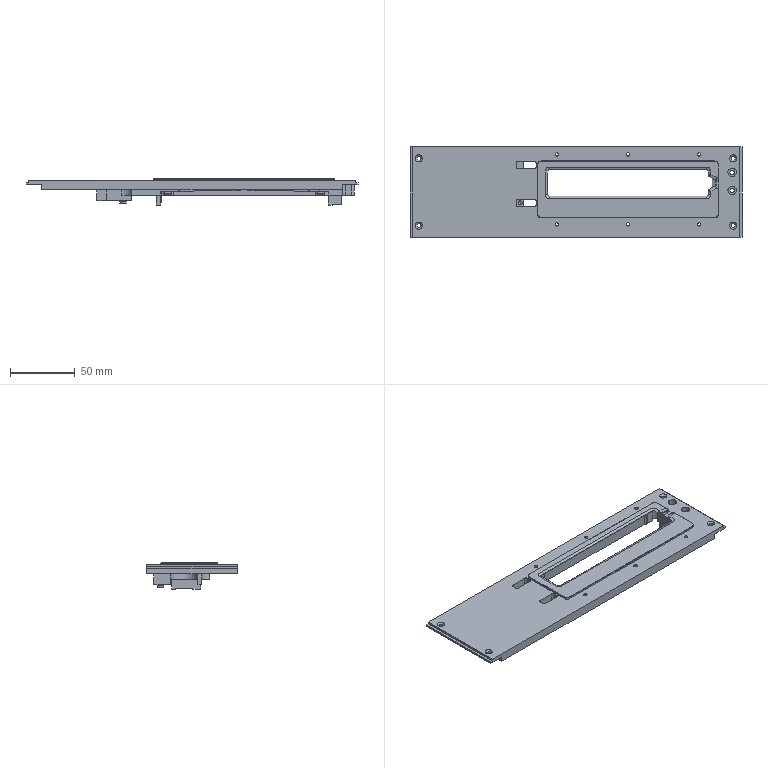NC program | NX | posted with a generic post | part box 256.6 x 70.3 x 20.422 mm
Lines 8840 to 9778 of 15201:
(HOLE_MILLING , TOOL : D3)
N17630 T03 M6
N17632 G54
N17634 G17 G0 G90 X120.7 Y15.17 S9500 M3
N17636 G43 Z30. H3
N17638 Z-0.9
N17640 G94 G3 X121.575 Y14.295 R0.875 F1250.
N17642 X122.45 Y15.17 R0.875
N17644 X122.45 Y15.17 Z-1.15 I-1.75 J0.
N17646 X122.45 Y15.17 Z-1.4 I-1.75 J0.
N17648 X122.45 Y15.17 Z-1.65 I-1.75 J0.
N17650 X122.45 Y15.17 Z-1.9 I-1.75 J0.
N17652 X122.45 Y15.17 Z-2.15 I-1.75 J0.
N17654 X122.45 Y15.17 Z-2.4 I-1.75 J0.
N17656 X122.45 Y15.17 Z-2.65 I-1.75 J0.
N17658 X122.45 Y15.17 Z-2.9 I-1.75 J0.
N17660 X122.45 Y15.17 Z-3.15 I-1.75 J0.
N17662 X122.45 Y15.17 Z-3.4 I-1.75 J0.
N17664 X122.45 Y15.17 Z-3.65 I-1.75 J0.
N17666 X122.45 Y15.17 Z-3.9 I-1.75 J0.
N17668 X122.45 Y15.17 Z-4.15 I-1.75 J0.
N17670 X122.45 Y15.17 Z-4.4 I-1.75 J0.
N17672 X122.45 Y15.17 Z-4.65 I-1.75 J0.
N17674 X122.45 Y15.17 Z-4.9 I-1.75 J0.
N17676 X122.45 Y15.17 Z-5.15 I-1.75 J0.
N17678 X122.45 Y15.17 Z-5.4 I-1.75 J0.
N17680 X122.45 Y15.17 Z-5.65 I-1.75 J0.
N17682 X122.45 Y15.17 Z-5.9 I-1.75 J0.
N17684 X122.45 Y15.17 Z-6.15 I-1.75 J0.
N17686 X122.45 Y15.17 Z-6.4 I-1.75 J0.
N17688 X122.45 Y15.17 Z-6.65 I-1.75 J0.
N17690 X122.45 Y15.17 Z-6.9 I-1.75 J0.
N17692 X122.45 Y15.17 Z-7.15 I-1.75 J0.
N17694 X122.45 Y15.17 Z-7.4 I-1.75 J0.
N17696 X122.45 Y15.17 Z-7.65 I-1.75 J0.
N17698 X122.45 Y15.17 Z-7.9 I-1.75 J0.
N17700 X122.45 Y15.17 Z-8.15 I-1.75 J0.
N17702 X122.45 Y15.17 Z-8.4 I-1.75 J0.
N17704 X122.45 Y15.17 Z-8.65 I-1.75 J0.
N17706 X122.441 Y14.994 Z-8.896 R-1.75
N17708 X120.876 Y16.911 R1.75
N17710 X122.441 Y14.994 R-1.75
N17712 X121.658 Y15.953 R0.875
N17714 X120.7 Y15.17 R0.875
N17716 G0 Z30.
N17718 Y1.17
N17720 Z-0.9
N17722 G3 X121.575 Y0.295 R0.875
N17724 X122.45 Y1.17 R0.875
N17726 X122.45 Y1.17 Z-1.15 I-1.75 J0.
N17728 X122.45 Y1.17 Z-1.4 I-1.75 J0.
N17730 X122.45 Y1.17 Z-1.65 I-1.75 J0.
N17732 X122.45 Y1.17 Z-1.9 I-1.75 J0.
N17734 X122.45 Y1.17 Z-2.15 I-1.75 J0.
N17736 X122.45 Y1.17 Z-2.4 I-1.75 J0.
N17738 X122.45 Y1.17 Z-2.65 I-1.75 J0.
N17740 X122.45 Y1.17 Z-2.9 I-1.75 J0.
N17742 X122.45 Y1.17 Z-3.15 I-1.75 J0.
N17744 X122.45 Y1.17 Z-3.4 I-1.75 J0.
N17746 X122.45 Y1.17 Z-3.65 I-1.75 J0.
N17748 X122.45 Y1.17 Z-3.9 I-1.75 J0.
N17750 X122.45 Y1.17 Z-4.15 I-1.75 J0.
N17752 X122.45 Y1.17 Z-4.4 I-1.75 J0.
N17754 X122.45 Y1.17 Z-4.65 I-1.75 J0.
N17756 X122.45 Y1.17 Z-4.9 I-1.75 J0.
N17758 X122.45 Y1.17 Z-5.15 I-1.75 J0.
N17760 X122.45 Y1.17 Z-5.4 I-1.75 J0.
N17762 X122.45 Y1.17 Z-5.65 I-1.75 J0.
N17764 X122.45 Y1.17 Z-5.9 I-1.75 J0.
N17766 X122.45 Y1.17 Z-6.15 I-1.75 J0.
N17768 X122.45 Y1.17 Z-6.4 I-1.75 J0.
N17770 X122.45 Y1.17 Z-6.65 I-1.75 J0.
N17772 X122.45 Y1.17 Z-6.9 I-1.75 J0.
N17774 X122.45 Y1.17 Z-7.15 I-1.75 J0.
N17776 X122.45 Y1.17 Z-7.4 I-1.75 J0.
N17778 X122.45 Y1.17 Z-7.65 I-1.75 J0.
N17780 X122.45 Y1.17 Z-7.9 I-1.75 J0.
N17782 X122.45 Y1.17 Z-8.15 I-1.75 J0.
N17784 X122.45 Y1.17 Z-8.4 I-1.75 J0.
N17786 X122.45 Y1.17 Z-8.65 I-1.75 J0.
N17788 X122.441 Y0.994 Z-8.896 R-1.75
N17790 X120.876 Y2.911 R1.75
N17792 X122.441 Y0.994 R-1.75
N17794 X121.658 Y1.953 R0.875
N17796 X120.7 Y1.17 R0.875
N17798 G0 Z30.
(ZLEVEL_PROFILE_COPY , TOOL : D3)
N17800 X-39.628 Y22.441
N17802 Z-0.4
N17804 G1 X-44.742 Z-0.668 F1000.
N17806 X-44.796 Y22.387 Z-0.672
N17808 Y19.448 Z-0.826
N17810 X-44.742 Y19.393 Z-0.83
N17812 X-32.356 Z-1.479
N17814 X-32.302 Y19.448 Z-1.483
N17816 Y22.387 Z-1.637
N17818 X-32.356 Y22.441 Z-1.641
N17820 X-32.402 Z-1.644
N17822 X-44.696 F1200.
N17824 X-44.751 Y22.436
N17826 X-44.791 Y22.396
N17828 X-44.796 Y22.341
N17830 Y19.493
N17832 X-44.791 Y19.438
N17834 X-44.751 Y19.398
N17836 X-44.696 Y19.393
N17838 X-32.402
N17840 X-32.347 Y19.398
N17842 X-32.307 Y19.438
N17844 X-32.302 Y19.493
N17846 Y22.341
N17848 X-32.307 Y22.396
N17850 X-32.347 Y22.436
N17852 X-32.402 Y22.441
N17854 X-44.521 Z-1.855
N17856 X-44.643 Y22.439 Z-1.857
N17858 X-44.731 Y22.427 Z-1.859
N17860 X-44.745 Y22.419
N17862 X-44.761 Y22.406 Z-1.86
N17864 X-44.78 Y22.381
N17866 X-44.793 Y22.306 Z-1.862
N17868 X-44.796 Y22.183 Z-1.864
N17870 Y20.837 Z-1.887
N17872 Y19.493
N17874 X-44.791 Y19.438
N17876 X-44.751 Y19.398
N17878 X-44.696 Y19.393
N17880 X-32.402
N17882 X-32.347 Y19.398
N17884 X-32.307 Y19.438
N17886 X-32.302 Y19.493
N17888 Y22.341
N17890 X-32.307 Y22.396
N17892 X-32.347 Y22.436
N17894 X-32.402 Y22.441
N17896 X-44.521 Z-2.099
N17898 X-44.643 Y22.439 Z-2.101
N17900 X-44.731 Y22.427 Z-2.102
N17902 X-44.747 Y22.419 Z-2.103
N17904 X-44.762 Y22.407
N17906 X-44.78 Y22.381 Z-2.104
N17908 X-44.793 Y22.306 Z-2.105
N17910 X-44.796 Y22.183 Z-2.107
N17912 Y20.837 Z-2.131
N17914 Y19.493
N17916 X-44.791 Y19.438
N17918 X-44.751 Y19.398
N17920 X-44.696 Y19.393
N17922 X-32.402
N17924 X-32.347 Y19.398
N17926 X-32.307 Y19.438
N17928 X-32.302 Y19.493
N17930 Y22.341
N17932 X-32.307 Y22.396
N17934 X-32.347 Y22.436
N17936 X-32.402 Y22.441
N17938 X-44.521 Z-2.342
N17940 X-44.643 Y22.439 Z-2.344
N17942 X-44.731 Y22.427 Z-2.346
N17944 X-44.747 Y22.419
N17946 X-44.762 Y22.407 Z-2.347
N17948 X-44.78 Y22.381
N17950 X-44.793 Y22.306 Z-2.349
N17952 X-44.796 Y22.183 Z-2.351
N17954 Y20.837 Z-2.374
N17956 Y19.493
N17958 X-44.791 Y19.438
N17960 X-44.751 Y19.398
N17962 X-44.696 Y19.393
N17964 X-32.402
N17966 X-32.347 Y19.398
N17968 X-32.307 Y19.438
N17970 X-32.302 Y19.493
N17972 Y22.341
N17974 X-32.307 Y22.396
N17976 X-32.347 Y22.436
N17978 X-32.402 Y22.441
N17980 X-44.521 Z-2.586
N17982 X-44.643 Y22.439 Z-2.588
N17984 X-44.731 Y22.426 Z-2.59
N17986 X-44.747 Y22.418
N17988 X-44.762 Y22.407
N17990 X-44.78 Y22.381 Z-2.591
N17992 X-44.793 Y22.306 Z-2.592
N17994 X-44.796 Y22.183 Z-2.594
N17996 Y20.837 Z-2.618
N17998 Y19.493
N18000 X-44.791 Y19.438
N18002 X-44.751 Y19.398
N18004 X-44.696 Y19.393
N18006 X-32.402
N18008 X-32.347 Y19.398
N18010 X-32.307 Y19.438
N18012 X-32.302 Y19.493
N18014 Y22.341
N18016 X-32.307 Y22.396
N18018 X-32.347 Y22.436
N18020 X-32.402 Y22.441
N18022 X-44.521 Z-2.829
N18024 X-44.643 Y22.439 Z-2.832
N18026 X-44.731 Y22.426 Z-2.833
N18028 X-44.747 Y22.418 Z-2.834
N18030 X-44.762 Y22.407
N18032 X-44.78 Y22.381 Z-2.835
N18034 X-44.793 Y22.306 Z-2.836
N18036 X-44.796 Y22.183 Z-2.838
N18038 Y20.837 Z-2.862
N18040 Y19.493
N18042 X-44.791 Y19.438
N18044 X-44.751 Y19.398
N18046 X-44.696 Y19.393
N18048 X-32.402
N18050 X-32.347 Y19.398
N18052 X-32.307 Y19.438
N18054 X-32.302 Y19.493
N18056 Y22.341
N18058 X-32.307 Y22.396
N18060 X-32.347 Y22.436
N18062 X-32.402 Y22.441
N18064 X-44.521 Z-3.073
N18066 X-44.643 Y22.439 Z-3.075
N18068 X-44.731 Y22.426 Z-3.077
N18070 X-44.747 Y22.418
N18072 X-44.762 Y22.407
N18074 X-44.78 Y22.381 Z-3.078
N18076 X-44.793 Y22.306 Z-3.079
N18078 X-44.796 Y22.183 Z-3.082
N18080 Y20.837 Z-3.105
N18082 Y19.493
N18084 X-44.791 Y19.438
N18086 X-44.751 Y19.398
N18088 X-44.696 Y19.393
N18090 X-32.402
N18092 X-32.347 Y19.398
N18094 X-32.307 Y19.438
N18096 X-32.302 Y19.493
N18098 Y22.341
N18100 X-32.307 Y22.396
N18102 X-32.347 Y22.436
N18104 X-32.402 Y22.441
N18106 X-44.521 Z-3.317
N18108 X-44.643 Y22.439 Z-3.319
N18110 X-44.731 Y22.426 Z-3.32
N18112 X-44.747 Y22.418 Z-3.321
N18114 X-44.762 Y22.407
N18116 X-44.78 Y22.381 Z-3.322
N18118 X-44.793 Y22.306 Z-3.323
N18120 X-44.796 Y22.183 Z-3.325
N18122 Y20.837 Z-3.349
N18124 Y19.493
N18126 X-44.791 Y19.438
N18128 X-44.751 Y19.398
N18130 X-44.696 Y19.393
N18132 X-32.402
N18134 X-32.347 Y19.398
N18136 X-32.307 Y19.438
N18138 X-32.302 Y19.493
N18140 Y22.341
N18142 X-32.307 Y22.396
N18144 X-32.347 Y22.436
N18146 X-32.402 Y22.441
N18148 X-44.521 Z-3.56
N18150 X-44.643 Y22.439 Z-3.562
N18152 X-44.731 Y22.426 Z-3.564
N18154 X-44.747 Y22.418
N18156 X-44.762 Y22.407 Z-3.565
N18158 X-44.78 Y22.381
N18160 X-44.793 Y22.306 Z-3.567
N18162 X-44.796 Y22.183 Z-3.569
N18164 Y20.837 Z-3.592
N18166 Y19.493
N18168 X-44.791 Y19.438
N18170 X-44.751 Y19.398
N18172 X-44.696 Y19.393
N18174 X-32.402
N18176 X-32.347 Y19.398
N18178 X-32.307 Y19.438
N18180 X-32.302 Y19.493
N18182 Y22.341
N18184 X-32.307 Y22.396
N18186 X-32.347 Y22.436
N18188 X-32.402 Y22.441
N18190 X-44.521 Z-3.804
N18192 X-44.643 Y22.439 Z-3.806
N18194 X-44.731 Y22.426 Z-3.807
N18196 X-44.747 Y22.418 Z-3.808
N18198 X-44.762 Y22.407
N18200 X-44.78 Y22.381 Z-3.809
N18202 X-44.793 Y22.306 Z-3.81
N18204 X-44.796 Y22.183 Z-3.812
N18206 Y20.837 Z-3.836
N18208 Y19.493
N18210 X-44.791 Y19.438
N18212 X-44.751 Y19.398
N18214 X-44.696 Y19.393
N18216 X-32.402
N18218 X-32.347 Y19.398
N18220 X-32.307 Y19.438
N18222 X-32.302 Y19.493
N18224 Y22.341
N18226 X-32.307 Y22.396
N18228 X-32.347 Y22.436
N18230 X-32.402 Y22.441
N18232 X-44.521 Z-4.047
N18234 X-44.643 Y22.439 Z-4.05
N18236 X-44.731 Y22.426 Z-4.051
N18238 X-44.747 Y22.418
N18240 X-44.762 Y22.407 Z-4.052
N18242 X-44.78 Y22.381 Z-4.053
N18244 X-44.793 Y22.306 Z-4.054
N18246 X-44.796 Y22.183 Z-4.056
N18248 Y20.837 Z-4.079
N18250 Y19.493
N18252 X-44.791 Y19.438
N18254 X-44.751 Y19.398
N18256 X-44.696 Y19.393
N18258 X-32.402
N18260 X-32.347 Y19.398
N18262 X-32.307 Y19.438
N18264 X-32.302 Y19.493
N18266 Y22.341
N18268 X-32.307 Y22.396
N18270 X-32.347 Y22.436
N18272 X-32.402 Y22.441
N18274 X-44.521 Z-4.291
N18276 X-44.643 Y22.439 Z-4.293
N18278 X-44.731 Y22.426 Z-4.295
N18280 X-44.747 Y22.418
N18282 X-44.762 Y22.407
N18284 X-44.78 Y22.381 Z-4.296
N18286 X-44.793 Y22.306 Z-4.297
N18288 X-44.796 Y22.183 Z-4.3
N18290 Y20.837 Z-4.323
N18292 Y19.493
N18294 X-44.791 Y19.438
N18296 X-44.751 Y19.398
N18298 X-44.696 Y19.393
N18300 X-32.402
N18302 X-32.347 Y19.398
N18304 X-32.307 Y19.438
N18306 X-32.302 Y19.493
N18308 Y22.341
N18310 X-32.307 Y22.396
N18312 X-32.347 Y22.436
N18314 X-32.402 Y22.441
N18316 X-44.521 Z-4.535
N18318 X-44.643 Y22.438 Z-4.537
N18320 X-44.731 Y22.426 Z-4.538
N18322 X-44.747 Y22.418 Z-4.539
N18324 X-44.762 Y22.407
N18326 X-44.779 Y22.381 Z-4.54
N18328 X-44.793 Y22.306 Z-4.541
N18330 X-44.796 Y22.183 Z-4.543
N18332 Y20.837 Z-4.567
N18334 Y19.493
N18336 X-44.791 Y19.438
N18338 X-44.751 Y19.398
N18340 X-44.696 Y19.393
N18342 X-32.402
N18344 X-32.347 Y19.398
N18346 X-32.307 Y19.438
N18348 X-32.302 Y19.493
N18350 Y22.341
N18352 X-32.307 Y22.396
N18354 X-32.347 Y22.436
N18356 X-32.402 Y22.441
N18358 X-44.521 Z-4.778
N18360 X-44.643 Y22.438 Z-4.78
N18362 X-44.732 Y22.427 Z-4.782
N18364 X-44.746 Y22.419
N18366 X-44.762 Y22.407 Z-4.783
N18368 X-44.779 Y22.381
N18370 X-44.793 Y22.306 Z-4.785
N18372 X-44.796 Y22.183 Z-4.787
N18374 Y20.837 Z-4.81
N18376 Y19.493
N18378 X-44.791 Y19.438
N18380 X-44.751 Y19.398
N18382 X-44.696 Y19.393
N18384 X-32.402
N18386 X-32.347 Y19.398
N18388 X-32.307 Y19.438
N18390 X-32.302 Y19.493
N18392 Y22.341
N18394 X-32.307 Y22.396
N18396 X-32.347 Y22.436
N18398 X-32.402 Y22.441
N18400 X-44.521 Z-5.022
N18402 X-44.643 Y22.438 Z-5.024
N18404 X-44.732 Y22.427 Z-5.025
N18406 X-44.746 Y22.419 Z-5.026
N18408 X-44.762 Y22.407
N18410 X-44.779 Y22.38 Z-5.027
N18412 X-44.793 Y22.306 Z-5.028
N18414 X-44.796 Y22.183 Z-5.03
N18416 Y20.837 Z-5.054
N18418 Y19.493
N18420 X-44.791 Y19.438
N18422 X-44.751 Y19.398
N18424 X-44.696 Y19.393
N18426 X-32.402
N18428 X-32.347 Y19.398
N18430 X-32.307 Y19.438
N18432 X-32.302 Y19.493
N18434 Y22.341
N18436 X-32.307 Y22.396
N18438 X-32.347 Y22.436
N18440 X-32.402 Y22.441
N18442 X-44.521 Z-5.265
N18444 X-44.643 Y22.438 Z-5.268
N18446 X-44.732 Y22.427 Z-5.269
N18448 X-44.746 Y22.419
N18450 X-44.762 Y22.407 Z-5.27
N18452 X-44.779 Y22.38
N18454 X-44.793 Y22.306 Z-5.272
N18456 X-44.796 Y22.183 Z-5.274
N18458 Y20.837 Z-5.297
N18460 Y19.493
N18462 X-44.791 Y19.438
N18464 X-44.751 Y19.398
N18466 X-44.696 Y19.393
N18468 X-32.402
N18470 X-32.347 Y19.398
N18472 X-32.307 Y19.438
N18474 X-32.302 Y19.493
N18476 Y22.341
N18478 X-32.307 Y22.396
N18480 X-32.347 Y22.436
N18482 X-32.402 Y22.441
N18484 X-44.521 Z-5.509
N18486 X-44.643 Y22.438 Z-5.511
N18488 X-44.732 Y22.427 Z-5.513
N18490 X-44.746 Y22.419
N18492 X-44.762 Y22.407
N18494 X-44.779 Y22.38 Z-5.514
N18496 X-44.792 Y22.306 Z-5.515
N18498 X-44.796 Y22.183 Z-5.518
N18500 Y20.837 Z-5.541
N18502 Y19.493
N18504 X-44.791 Y19.438
N18506 X-44.751 Y19.398
N18508 X-44.696 Y19.393
N18510 X-32.402
N18512 X-32.347 Y19.398
N18514 X-32.307 Y19.438
N18516 X-32.302 Y19.493
N18518 Y22.341
N18520 X-32.307 Y22.396
N18522 X-32.347 Y22.436
N18524 X-32.402 Y22.441
N18526 X-44.521 Z-5.753
N18528 X-44.643 Y22.438 Z-5.755
N18530 X-44.732 Y22.427 Z-5.756
N18532 X-44.746 Y22.419 Z-5.757
N18534 X-44.762 Y22.407
N18536 X-44.779 Y22.38 Z-5.758
N18538 X-44.792 Y22.306 Z-5.759
N18540 X-44.796 Y22.183 Z-5.761
N18542 Y20.837 Z-5.785
N18544 Y19.493
N18546 X-44.791 Y19.438
N18548 X-44.751 Y19.398
N18550 X-44.696 Y19.393
N18552 X-32.402
N18554 X-32.347 Y19.398
N18556 X-32.307 Y19.438
N18558 X-32.302 Y19.493
N18560 Y22.341
N18562 X-32.307 Y22.396
N18564 X-32.347 Y22.436
N18566 X-32.402 Y22.441
N18568 X-44.521 Z-5.996
N18570 X-44.643 Y22.438 Z-5.998
N18572 X-44.732 Y22.427 Z-6.
N18574 X-44.746 Y22.419
N18576 X-44.762 Y22.406 Z-6.001
N18578 X-44.779 Y22.38
N18580 X-44.792 Y22.306 Z-6.003
N18582 X-44.796 Y22.183 Z-6.005
N18584 Y20.837 Z-6.028
N18586 Y19.493
N18588 X-44.791 Y19.438
N18590 X-44.751 Y19.398
N18592 X-44.696 Y19.393
N18594 X-32.402
N18596 X-32.347 Y19.398
N18598 X-32.307 Y19.438
N18600 X-32.302 Y19.493
N18602 Y22.341
N18604 X-32.307 Y22.396
N18606 X-32.347 Y22.436
N18608 X-32.402 Y22.441
N18610 X-44.521 Z-6.24
N18612 X-44.643 Y22.438 Z-6.242
N18614 X-44.732 Y22.427 Z-6.243
N18616 X-44.746 Y22.419 Z-6.244
N18618 X-44.762 Y22.406
N18620 X-44.779 Y22.38 Z-6.245
N18622 X-44.792 Y22.306 Z-6.246
N18624 X-44.796 Y22.183 Z-6.248
N18626 Y20.837 Z-6.272
N18628 Y19.493
N18630 X-44.791 Y19.438
N18632 X-44.751 Y19.398
N18634 X-44.696 Y19.393
N18636 X-32.402
N18638 X-32.347 Y19.398
N18640 X-32.307 Y19.438
N18642 X-32.302 Y19.493
N18644 Y22.341
N18646 X-32.307 Y22.396
N18648 X-32.347 Y22.436
N18650 X-32.402 Y22.441
N18652 X-44.521 Z-6.483
N18654 X-44.643 Y22.438 Z-6.485
N18656 X-44.732 Y22.427 Z-6.487
N18658 X-44.746 Y22.419
N18660 X-44.762 Y22.406 Z-6.488
N18662 X-44.779 Y22.38
N18664 X-44.792 Y22.306 Z-6.49
N18666 X-44.796 Y22.183 Z-6.492
N18668 Y20.837 Z-6.515
N18670 Y19.493
N18672 X-44.791 Y19.438
N18674 X-44.751 Y19.398
N18676 X-44.696 Y19.393
N18678 X-32.402
N18680 X-32.347 Y19.398
N18682 X-32.307 Y19.438
N18684 X-32.302 Y19.493
N18686 Y22.341
N18688 X-32.307 Y22.396
N18690 X-32.347 Y22.436
N18692 X-32.402 Y22.441
N18694 X-44.521 Z-6.727
N18696 X-44.643 Y22.438 Z-6.729
N18698 X-44.732 Y22.427 Z-6.731
N18700 X-44.746 Y22.419
N18702 X-44.761 Y22.406
N18704 X-44.779 Y22.38 Z-6.732
N18706 X-44.792 Y22.306 Z-6.733
N18708 X-44.796 Y22.183 Z-6.735
N18710 Y20.837 Z-6.759
N18712 Y19.493
N18714 X-44.791 Y19.438
N18716 X-44.751 Y19.398
N18718 X-44.696 Y19.393
N18720 X-32.402
N18722 X-32.347 Y19.398
N18724 X-32.307 Y19.438
N18726 X-32.302 Y19.493
N18728 Y22.341
N18730 X-32.307 Y22.396
N18732 X-32.347 Y22.436
N18734 X-32.402 Y22.441
N18736 X-44.521 Z-6.97
N18738 X-44.643 Y22.438 Z-6.973
N18740 X-44.732 Y22.427 Z-6.974
N18742 X-44.746 Y22.418
N18744 X-44.761 Y22.406 Z-6.975
N18746 X-44.779 Y22.38 Z-6.976
N18748 X-44.792 Y22.306 Z-6.977
N18750 X-44.796 Y22.183 Z-6.979
N18752 Y20.837 Z-7.003
N18754 Y19.493
N18756 X-44.791 Y19.438
N18758 X-44.751 Y19.398
N18760 X-44.696 Y19.393
N18762 X-32.402
N18764 X-32.347 Y19.398
N18766 X-32.307 Y19.438
N18768 X-32.302 Y19.493
N18770 Y22.341
N18772 X-32.307 Y22.396
N18774 X-32.347 Y22.436
N18776 X-32.402 Y22.441
N18778 X-44.521 Z-7.214
N18780 X-44.643 Y22.438 Z-7.216
N18782 X-44.732 Y22.427 Z-7.218
N18784 X-44.746 Y22.418
N18786 X-44.761 Y22.406
N18788 X-44.779 Y22.38 Z-7.219
N18790 X-44.792 Y22.306 Z-7.22
N18792 X-44.796 Y22.183 Z-7.223
N18794 Y20.837 Z-7.246
N18796 Y19.493
N18798 X-44.791 Y19.438
N18800 X-44.751 Y19.398
N18802 X-44.696 Y19.393
N18804 X-32.402
N18806 X-32.347 Y19.398
N18808 X-32.307 Y19.438
N18810 X-32.302 Y19.493
N18812 Y22.341
N18814 X-32.307 Y22.396
N18816 X-32.347 Y22.436
N18818 X-32.402 Y22.441
N18820 X-44.521 Z-7.458
N18822 X-44.643 Y22.438 Z-7.46
N18824 X-44.732 Y22.426 Z-7.461
N18826 X-44.746 Y22.418 Z-7.462
N18828 X-44.761 Y22.406
N18830 X-44.779 Y22.38 Z-7.463
N18832 X-44.792 Y22.306 Z-7.464
N18834 X-44.796 Y22.183 Z-7.466
N18836 Y20.837 Z-7.49
N18838 Y19.493
N18840 X-44.791 Y19.438
N18842 X-44.751 Y19.398
N18844 X-44.696 Y19.393
N18846 X-32.402
N18848 X-32.347 Y19.398
N18850 X-32.307 Y19.438
N18852 X-32.302 Y19.493
N18854 Y22.341
N18856 X-32.307 Y22.396
N18858 X-32.347 Y22.436
N18860 X-32.402 Y22.441
N18862 X-44.521 Z-7.701
N18864 X-44.643 Y22.438 Z-7.703
N18866 X-44.731 Y22.426 Z-7.705
N18868 X-44.746 Y22.418
N18870 X-44.761 Y22.406 Z-7.706
N18872 X-44.779 Y22.38
N18874 X-44.792 Y22.306 Z-7.708
N18876 X-44.796 Y22.183 Z-7.71
N18878 Y20.837 Z-7.733
N18880 Y19.493
N18882 X-44.791 Y19.438
N18884 X-44.751 Y19.398
N18886 X-44.696 Y19.393
N18888 X-32.402
N18890 X-32.347 Y19.398
N18892 X-32.307 Y19.438
N18894 X-32.302 Y19.493
N18896 Y22.341
N18898 X-32.307 Y22.396
N18900 X-32.347 Y22.436
N18902 X-32.402 Y22.441
N18904 X-44.521 Z-7.945
N18906 X-44.643 Y22.438 Z-7.947
N18908 X-44.731 Y22.426 Z-7.948
N18910 X-44.746 Y22.418 Z-7.949
N18912 X-44.761 Y22.406
N18914 X-44.779 Y22.38 Z-7.95
N18916 X-44.792 Y22.306 Z-7.951
N18918 X-44.796 Y22.183 Z-7.953
N18920 Y20.837 Z-7.977
N18922 Y19.493
N18924 X-44.791 Y19.438
N18926 X-44.751 Y19.398
N18928 X-44.696 Y19.393
N18930 X-32.402
N18932 X-32.347 Y19.398
N18934 X-32.307 Y19.438
N18936 X-32.302 Y19.493
N18938 Y22.341
N18940 X-32.307 Y22.396
N18942 X-32.347 Y22.436
N18944 X-32.402 Y22.441
N18946 X-44.521 Z-8.188
N18948 X-44.643 Y22.438 Z-8.191
N18950 X-44.731 Y22.426 Z-8.192
N18952 X-44.746 Y22.418
N18954 X-44.761 Y22.406 Z-8.193
N18956 X-44.779 Y22.38
N18958 X-44.792 Y22.306 Z-8.195
N18960 X-44.796 Y22.183 Z-8.197
N18962 Y20.837 Z-8.22
N18964 Y19.493
N18966 X-44.791 Y19.438
N18968 X-44.751 Y19.398
N18970 X-44.696 Y19.393
N18972 X-32.402
N18974 X-32.347 Y19.398
N18976 X-32.307 Y19.438
N18978 X-32.302 Y19.493
N18980 Y22.341
N18982 X-32.307 Y22.396
N18984 X-32.347 Y22.436
N18986 X-32.402 Y22.441
N18988 X-44.521 Z-8.432
N18990 X-44.643 Y22.438 Z-8.434
N18992 X-44.731 Y22.426 Z-8.436
N18994 X-44.746 Y22.418
N18996 X-44.761 Y22.406
N18998 X-44.779 Y22.38 Z-8.437
N19000 X-44.792 Y22.306 Z-8.438
N19002 X-44.796 Y22.183 Z-8.441
N19004 Y20.837 Z-8.464
N19006 Y19.493
N19008 X-44.791 Y19.438
N19010 X-44.751 Y19.398
N19012 X-44.696 Y19.393
N19014 X-32.402
N19016 X-32.347 Y19.398
N19018 X-32.307 Y19.438
N19020 X-32.302 Y19.493
N19022 Y22.341
N19024 X-32.307 Y22.396
N19026 X-32.347 Y22.436
N19028 X-32.402 Y22.441
N19030 X-44.521 Z-8.676
N19032 X-44.643 Y22.438 Z-8.678
N19034 X-44.731 Y22.426 Z-8.679
N19036 X-44.746 Y22.418 Z-8.68
N19038 X-44.761 Y22.406
N19040 X-44.779 Y22.38 Z-8.681
N19042 X-44.792 Y22.306 Z-8.682
N19044 X-44.796 Y22.183 Z-8.684
N19046 Y20.837 Z-8.708
N19048 Y19.493
N19050 X-44.791 Y19.438
N19052 X-44.751 Y19.398
N19054 X-44.696 Y19.393
N19056 X-32.402
N19058 X-32.347 Y19.398
N19060 X-32.307 Y19.438
N19062 X-32.302 Y19.493
N19064 Y22.341
N19066 X-32.307 Y22.396
N19068 X-32.347 Y22.436
N19070 X-32.402 Y22.441
N19072 X-44.521 Z-8.919
N19074 X-44.643 Y22.438 Z-8.921
N19076 X-44.731 Y22.426 Z-8.923
N19078 X-44.746 Y22.418
N19080 X-44.761 Y22.406 Z-8.924
N19082 X-44.779 Y22.38
N19084 X-44.792 Y22.306 Z-8.926
N19086 X-44.796 Y22.183 Z-8.928
N19088 Y20.837 Z-8.951
N19090 Y19.493
N19092 X-44.791 Y19.438
N19094 X-44.751 Y19.398
N19096 X-44.696 Y19.393
N19098 X-32.402
N19100 X-32.347 Y19.398
N19102 X-32.307 Y19.438
N19104 X-32.302 Y19.493
N19106 Y22.341
N19108 X-32.307 Y22.396
N19110 X-32.347 Y22.436
N19112 X-32.402 Y22.441
N19114 X-44.521 Z-9.163
N19116 X-44.643 Y22.438 Z-9.165
N19118 X-44.731 Y22.426 Z-9.166
N19120 X-44.746 Y22.418 Z-9.167
N19122 X-44.761 Y22.406
N19124 X-44.779 Y22.38 Z-9.168
N19126 X-44.792 Y22.306 Z-9.169
N19128 X-44.796 Y22.183 Z-9.171
N19130 Y20.837 Z-9.195
N19132 Y19.493
N19134 X-44.791 Y19.438
N19136 X-44.751 Y19.398
N19138 X-44.696 Y19.393
N19140 X-32.402
N19142 X-32.347 Y19.398
N19144 X-32.307 Y19.438
N19146 X-32.302 Y19.493
N19148 Y22.341
N19150 X-32.307 Y22.396
N19152 X-32.347 Y22.436
N19154 X-32.402 Y22.441
N19156 X-44.528 Z-9.406
N19158 X-44.674 Y22.435 Z-9.409
N19160 X-44.738 Y22.423 Z-9.41
N19162 X-44.759 Y22.409 Z-9.411
N19164 X-44.775 Y22.386
N19166 X-44.782 Y22.374 Z-9.412
N19168 X-44.791 Y22.312 Z-9.413
N19170 X-44.796 Y22.18 Z-9.415
N19172 Y20.725 Z-9.44
N19174 Y19.493
N19176 X-44.791 Y19.438
N19178 X-44.751 Y19.398
N19180 X-44.696 Y19.393
N19182 X-32.402
N19184 X-32.347 Y19.398
N19186 X-32.307 Y19.438
N19188 X-32.302 Y19.493
N19190 Y22.341
N19192 X-32.307 Y22.396
N19194 X-32.347 Y22.436
N19196 X-32.402 Y22.441
N19198 X-44.528 Z-9.652
N19200 X-44.674 Y22.435 Z-9.654
N19202 X-44.738 Y22.423 Z-9.656
N19204 X-44.759 Y22.408
N19206 X-44.775 Y22.386 Z-9.657
N19208 X-44.782 Y22.374
N19210 X-44.791 Y22.312 Z-9.658
N19212 X-44.796 Y22.18 Z-9.66
N19214 Y20.725 Z-9.686
N19216 Y19.493
N19218 X-44.791 Y19.438
N19220 X-44.751 Y19.398
N19222 X-44.696 Y19.393
N19224 X-32.402
N19226 X-32.347 Y19.398
N19228 X-32.307 Y19.438
N19230 X-32.302 Y19.493
N19232 Y22.341
N19234 X-32.307 Y22.396
N19236 X-32.347 Y22.436
N19238 X-32.402 Y22.441
N19240 X-44.528 Z-9.898
N19242 X-44.674 Y22.435 Z-9.9
N19244 X-44.738 Y22.423 Z-9.901
N19246 X-44.759 Y22.408 Z-9.902
N19248 X-44.776 Y22.386
N19250 X-44.782 Y22.374 Z-9.903
N19252 X-44.791 Y22.312 Z-9.904
N19254 X-44.796 Y22.18 Z-9.906
N19256 Y20.725 Z-9.931
N19258 Y19.493
N19260 X-44.791 Y19.438
N19262 X-44.751 Y19.398
N19264 X-44.696 Y19.393
N19266 X-32.402
N19268 X-32.347 Y19.398
N19270 X-32.307 Y19.438
N19272 X-32.302 Y19.493
N19274 Y22.341
N19276 X-32.307 Y22.396
N19278 X-32.347 Y22.436
N19280 X-32.402 Y22.441
N19282 X-44.528 Z-10.143
N19284 X-44.674 Y22.435 Z-10.146
N19286 X-44.738 Y22.423 Z-10.147
N19288 X-44.759 Y22.408
N19290 X-44.776 Y22.386 Z-10.148
N19292 X-44.782 Y22.374
N19294 X-44.791 Y22.312 Z-10.149
N19296 X-44.796 Y22.18 Z-10.152
N19298 Y20.725 Z-10.177
N19300 Y19.493
N19302 X-44.791 Y19.438
N19304 X-44.751 Y19.398
N19306 X-44.696 Y19.393
N19308 X-32.402
N19310 X-32.347 Y19.398
N19312 X-32.307 Y19.438
N19314 X-32.302 Y19.493
N19316 Y22.341
N19318 X-32.307 Y22.396
N19320 X-32.347 Y22.436
N19322 X-32.402 Y22.441
N19324 X-44.528 Z-10.389
N19326 X-44.674 Y22.435 Z-10.391
N19328 X-44.738 Y22.423 Z-10.392
N19330 X-44.759 Y22.408 Z-10.393
N19332 X-44.776 Y22.386
N19334 X-44.782 Y22.374 Z-10.394
N19336 X-44.791 Y22.312 Z-10.395
N19338 X-44.796 Y22.18 Z-10.397
N19340 Y20.725 Z-10.422
N19342 Y19.493
N19344 X-44.791 Y19.438
N19346 X-44.751 Y19.398
N19348 X-44.696 Y19.393
N19350 X-32.402
N19352 X-32.347 Y19.398
N19354 X-32.307 Y19.438
N19356 X-32.302 Y19.493
N19358 Y22.341
N19360 X-32.307 Y22.396
N19362 X-32.347 Y22.436
N19364 X-32.402 Y22.441
N19366 X-44.528 Z-10.634
N19368 X-44.674 Y22.435 Z-10.637
N19370 X-44.738 Y22.423 Z-10.638
N19372 X-44.759 Y22.408
N19374 X-44.776 Y22.386 Z-10.639
N19376 X-44.782 Y22.374
N19378 X-44.791 Y22.312 Z-10.64
N19380 X-44.796 Y22.18 Z-10.643
N19382 Y20.725 Z-10.668
N19384 Y19.493
N19386 X-44.791 Y19.438
N19388 X-44.751 Y19.398
N19390 X-44.696 Y19.393
N19392 X-32.402
N19394 X-32.347 Y19.398
N19396 X-32.307 Y19.438
N19398 X-32.302 Y19.493
N19400 Y22.341
N19402 X-32.307 Y22.396
N19404 X-32.347 Y22.436
N19406 X-32.402 Y22.441
N19408 X-44.696
N19410 X-44.751 Y22.436
N19412 X-44.791 Y22.396
N19414 X-44.796 Y22.341
N19416 Y20.725
N19418 G3 X-44.646 Y20.465 R0.3
N19420 G1 X-44.196 Y20.206
N19422 Z-10.368
N19424 G0 Z30.
(ZLEVEL_PROFILE_COPY_COPY , TOOL : D3)
N19426 X-37.469 Y-10.041
N19428 Z-0.4
N19430 G1 X-32.402 Z-0.666 F1000.
N19432 X-32.356 Z-0.668
N19434 X-32.302 Y-9.987 Z-0.672
N19436 Y-9.941 Z-0.674
N19438 Y-7.048 Z-0.826
N19440 X-32.356 Y-6.994 Z-0.83
N19442 X-44.742 Z-1.479
N19444 X-44.796 Y-7.048 Z-1.483
N19446 Y-9.987 Z-1.637
N19448 X-44.742 Y-10.041 Z-1.641
N19450 X-44.696 Z-1.644
N19452 X-32.402 F1200.
N19454 X-32.347 Y-10.036
N19456 X-32.307 Y-9.996
N19458 X-32.302 Y-9.941
N19460 Y-7.094
N19462 X-32.307 Y-7.039
N19464 X-32.347 Y-6.998
N19466 X-32.402 Y-6.994
N19468 X-44.696
N19470 X-44.751 Y-6.998
N19472 X-44.791 Y-7.039
N19474 X-44.796 Y-7.094
N19476 Y-9.941
N19478 X-44.791 Y-9.996
N19480 X-44.751 Y-10.036
N19482 X-44.696 Y-10.041
N19484 X-32.454 Z-1.857
N19486 X-32.361 Y-10.033 Z-1.859
N19488 X-32.348 Y-10.025